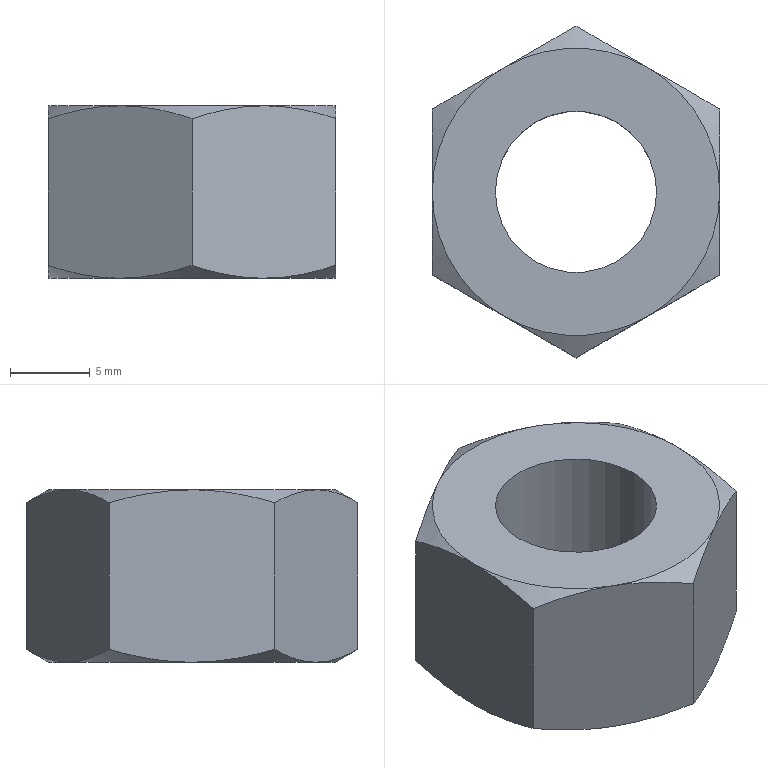Part | SolidWorks | features Cut 2, Extrusion 1 | 1 solid | 22 faces | box 18 x 20.785 x 10.8 mm | volume 2151 mm3 | cone 12 | plane 8 | cylinder 2 | commonest cylinder face diameters 10.106 x2
STEP:
#1=CARTESIAN_POINT('',(-5.053,0.,10.8));
#2=VERTEX_POINT('',#1);
#3=CARTESIAN_POINT('',(5.053,0.,10.8));
#4=VERTEX_POINT('',#3);
#5=CARTESIAN_POINT('',(0.,0.,10.8));
#6=DIRECTION('',(0.,0.,1.));
#7=DIRECTION('',(1.,0.,0.));
#8=AXIS2_PLACEMENT_3D('',#5,#6,#7);
#9=CIRCLE('',#8,5.053);
#10=EDGE_CURVE('',#2,#4,#9,.T.);
#11=ORIENTED_EDGE('',*,*,#10,.T.);
#12=CARTESIAN_POINT('',(5.053,0.,0.));
#13=VERTEX_POINT('',#12);
#14=CARTESIAN_POINT('',(5.053,0.,10.8));
#15=DIRECTION('',(0.,0.,-1.));
#16=VECTOR('',#15,1000.);
#17=LINE('',#14,#16);
#18=EDGE_CURVE('',#4,#13,#17,.T.);
#19=ORIENTED_EDGE('',*,*,#18,.T.);
#20=CARTESIAN_POINT('',(-5.053,0.,0.));
#21=VERTEX_POINT('',#20);
#22=CARTESIAN_POINT('',(0.,0.,0.));
#23=DIRECTION('',(0.,0.,1.));
#24=DIRECTION('',(1.,0.,0.));
#25=AXIS2_PLACEMENT_3D('',#22,#23,#24);
#26=CIRCLE('',#25,5.053);
#27=EDGE_CURVE('',#21,#13,#26,.T.);
#28=ORIENTED_EDGE('',*,*,#27,.F.);
#29=CARTESIAN_POINT('',(-5.053,0.,10.8));
#30=DIRECTION('',(0.,0.,-1.));
#31=VECTOR('',#30,1000.);
#32=LINE('',#29,#31);
#33=EDGE_CURVE('',#2,#21,#32,.T.);
#34=ORIENTED_EDGE('',*,*,#33,.F.);
#35=EDGE_LOOP('',(#11,#19,#28,#34));
#36=FACE_OUTER_BOUND('',#35,.T.);
#37=CARTESIAN_POINT('',(0.,0.,10.8));
#38=DIRECTION('',(0.,0.,-1.));
#39=DIRECTION('',(-1.,0.,0.));
#40=AXIS2_PLACEMENT_3D('',#37,#38,#39);
#41=CYLINDRICAL_SURFACE('',#40,5.053);
#42=ADVANCED_FACE('',(#36),#41,.F.);
#43=CARTESIAN_POINT('',(9.,5.196,9.996));
#44=VERTEX_POINT('',#43);
#45=CARTESIAN_POINT('',(4.5,7.794,10.8));
#46=VERTEX_POINT('',#45);
#47=CARTESIAN_POINT('',(9.,5.196,9.996));
#48=CARTESIAN_POINT('',(8.264,5.621,10.242));
#49=CARTESIAN_POINT('',(7.522,6.049,10.444));
#50=CARTESIAN_POINT('',(6.024,6.914,10.723));
#51=CARTESIAN_POINT('',(5.267,7.352,10.8));
#52=CARTESIAN_POINT('',(4.5,7.794,10.8));
#53=B_SPLINE_CURVE_WITH_KNOTS('',3,(#47,#48,#49,#50,#51,#52),.UNSPECIFIED.,.F.,.F.,(4,2,4),(0.000000238,0.002629,0.005258),.UNSPECIFIED.);
#54=EDGE_CURVE('',#44,#46,#53,.T.);
#55=ORIENTED_EDGE('',*,*,#54,.F.);
#56=CARTESIAN_POINT('',(9.,5.196,0.8038));
#57=VERTEX_POINT('',#56);
#58=CARTESIAN_POINT('',(9.,5.196,10.8));
#59=DIRECTION('',(0.,0.,-1.));
#60=VECTOR('',#59,1000.);
#61=LINE('',#58,#60);
#62=EDGE_CURVE('',#44,#57,#61,.T.);
#63=ORIENTED_EDGE('',*,*,#62,.T.);
#64=CARTESIAN_POINT('',(4.5,7.794,0.));
#65=VERTEX_POINT('',#64);
#66=CARTESIAN_POINT('',(4.5,7.794,0.));
#67=CARTESIAN_POINT('',(4.882,7.574,0.));
#68=CARTESIAN_POINT('',(5.266,7.352,0.019));
#69=CARTESIAN_POINT('',(6.024,6.914,0.09253));
#70=CARTESIAN_POINT('',(6.401,6.697,0.147));
#71=CARTESIAN_POINT('',(7.525,6.048,0.357));
#72=CARTESIAN_POINT('',(8.266,5.62,0.5591));
#73=CARTESIAN_POINT('',(9.,5.196,0.8038));
#74=B_SPLINE_CURVE_WITH_KNOTS('',3,(#66,#67,#68,#69,#70,#71,#72,#73),.UNSPECIFIED.,.F.,.F.,(4,2,2,4),(0.005258,0.006567,0.007877,0.0105),.UNSPECIFIED.);
#75=EDGE_CURVE('',#65,#57,#74,.T.);
#76=ORIENTED_EDGE('',*,*,#75,.F.);
#77=CARTESIAN_POINT('',(0.,10.392,0.8038));
#78=VERTEX_POINT('',#77);
#79=CARTESIAN_POINT('',(0.,10.392,0.8038));
#80=CARTESIAN_POINT('',(0.7361,9.967,0.5585));
#81=CARTESIAN_POINT('',(1.478,9.539,0.3563));
#82=CARTESIAN_POINT('',(2.976,8.674,0.07661));
#83=CARTESIAN_POINT('',(3.733,8.237,0.));
#84=CARTESIAN_POINT('',(4.5,7.794,0.));
#85=B_SPLINE_CURVE_WITH_KNOTS('',3,(#79,#80,#81,#82,#83,#84),.UNSPECIFIED.,.F.,.F.,(4,2,4),(0.000000238,0.002629,0.005258),.UNSPECIFIED.);
#86=EDGE_CURVE('',#78,#65,#85,.T.);
#87=ORIENTED_EDGE('',*,*,#86,.F.);
#88=CARTESIAN_POINT('',(0.,10.392,9.996));
#89=VERTEX_POINT('',#88);
#90=CARTESIAN_POINT('',(0.,10.392,10.8));
#91=DIRECTION('',(0.,0.,-1.));
#92=VECTOR('',#91,1000.);
#93=LINE('',#90,#92);
#94=EDGE_CURVE('',#89,#78,#93,.T.);
#95=ORIENTED_EDGE('',*,*,#94,.F.);
#96=CARTESIAN_POINT('',(4.5,7.794,10.8));
#97=CARTESIAN_POINT('',(4.118,8.015,10.8));
#98=CARTESIAN_POINT('',(3.734,8.236,10.781));
#99=CARTESIAN_POINT('',(2.976,8.674,10.707));
#100=CARTESIAN_POINT('',(2.599,8.892,10.653));
#101=CARTESIAN_POINT('',(1.475,9.541,10.443));
#102=CARTESIAN_POINT('',(0.7343,9.968,10.241));
#103=CARTESIAN_POINT('',(0.,10.392,9.996));
#104=B_SPLINE_CURVE_WITH_KNOTS('',3,(#96,#97,#98,#99,#100,#101,#102,#103),.UNSPECIFIED.,.F.,.F.,(4,2,2,4),(0.005258,0.006567,0.007877,0.0105),.UNSPECIFIED.);
#105=EDGE_CURVE('',#46,#89,#104,.T.);
#106=ORIENTED_EDGE('',*,*,#105,.F.);
#107=EDGE_LOOP('',(#55,#63,#76,#87,#95,#106));
#108=FACE_OUTER_BOUND('',#107,.T.);
#109=CARTESIAN_POINT('',(9.,5.196,10.8));
#110=DIRECTION('',(-0.5,-0.866,0.));
#111=DIRECTION('',(0.866,-0.5,0.));
#112=AXIS2_PLACEMENT_3D('',#109,#110,#111);
#113=PLANE('',#112);
#114=ADVANCED_FACE('',(#108),#113,.F.);
#115=CARTESIAN_POINT('',(-4.5,7.794,10.8));
#116=VERTEX_POINT('',#115);
#117=CARTESIAN_POINT('',(0.,10.392,9.996));
#118=CARTESIAN_POINT('',(-0.7361,9.967,10.242));
#119=CARTESIAN_POINT('',(-1.478,9.539,10.444));
#120=CARTESIAN_POINT('',(-2.976,8.674,10.723));
#121=CARTESIAN_POINT('',(-3.733,8.237,10.8));
#122=CARTESIAN_POINT('',(-4.5,7.794,10.8));
#123=B_SPLINE_CURVE_WITH_KNOTS('',3,(#117,#118,#119,#120,#121,#122),.UNSPECIFIED.,.F.,.F.,(4,2,4),(0.000000238,0.002629,0.005258),.UNSPECIFIED.);
#124=EDGE_CURVE('',#89,#116,#123,.T.);
#125=ORIENTED_EDGE('',*,*,#124,.F.);
#126=ORIENTED_EDGE('',*,*,#94,.T.);
#127=CARTESIAN_POINT('',(-4.5,7.794,0.));
#128=VERTEX_POINT('',#127);
#129=CARTESIAN_POINT('',(-4.5,7.794,0.));
#130=CARTESIAN_POINT('',(-4.118,8.015,0.));
#131=CARTESIAN_POINT('',(-3.734,8.236,0.019));
#132=CARTESIAN_POINT('',(-2.976,8.674,0.09253));
#133=CARTESIAN_POINT('',(-2.599,8.892,0.147));
#134=CARTESIAN_POINT('',(-1.475,9.541,0.357));
#135=CARTESIAN_POINT('',(-0.7343,9.968,0.5591));
#136=CARTESIAN_POINT('',(0.,10.392,0.8038));
#137=B_SPLINE_CURVE_WITH_KNOTS('',3,(#129,#130,#131,#132,#133,#134,#135,#136),.UNSPECIFIED.,.F.,.F.,(4,2,2,4),(0.005258,0.006567,0.007877,0.0105),.UNSPECIFIED.);
#138=EDGE_CURVE('',#128,#78,#137,.T.);
#139=ORIENTED_EDGE('',*,*,#138,.F.);
#140=CARTESIAN_POINT('',(-9.,5.196,0.8038));
#141=VERTEX_POINT('',#140);
#142=CARTESIAN_POINT('',(-9.,5.196,0.8038));
#143=CARTESIAN_POINT('',(-8.264,5.621,0.5585));
#144=CARTESIAN_POINT('',(-7.522,6.049,0.3563));
#145=CARTESIAN_POINT('',(-6.024,6.914,0.07661));
#146=CARTESIAN_POINT('',(-5.267,7.352,0.));
#147=CARTESIAN_POINT('',(-4.5,7.794,0.));
#148=B_SPLINE_CURVE_WITH_KNOTS('',3,(#142,#143,#144,#145,#146,#147),.UNSPECIFIED.,.F.,.F.,(4,2,4),(0.000000238,0.002629,0.005258),.UNSPECIFIED.);
#149=EDGE_CURVE('',#141,#128,#148,.T.);
#150=ORIENTED_EDGE('',*,*,#149,.F.);
#151=CARTESIAN_POINT('',(-9.,5.196,9.996));
#152=VERTEX_POINT('',#151);
#153=CARTESIAN_POINT('',(-9.,5.196,10.8));
#154=DIRECTION('',(0.,0.,-1.));
#155=VECTOR('',#154,1000.);
#156=LINE('',#153,#155);
#157=EDGE_CURVE('',#152,#141,#156,.T.);
#158=ORIENTED_EDGE('',*,*,#157,.F.);
#159=CARTESIAN_POINT('',(-4.5,7.794,10.8));
#160=CARTESIAN_POINT('',(-4.882,7.574,10.8));
#161=CARTESIAN_POINT('',(-5.266,7.352,10.781));
#162=CARTESIAN_POINT('',(-6.024,6.914,10.707));
#163=CARTESIAN_POINT('',(-6.401,6.697,10.653));
#164=CARTESIAN_POINT('',(-7.525,6.048,10.443));
#165=CARTESIAN_POINT('',(-8.266,5.62,10.241));
#166=CARTESIAN_POINT('',(-9.,5.196,9.996));
#167=B_SPLINE_CURVE_WITH_KNOTS('',3,(#159,#160,#161,#162,#163,#164,#165,#166),.UNSPECIFIED.,.F.,.F.,(4,2,2,4),(0.005258,0.006567,0.007877,0.0105),.UNSPECIFIED.);
#168=EDGE_CURVE('',#116,#152,#167,.T.);
#169=ORIENTED_EDGE('',*,*,#168,.F.);
#170=EDGE_LOOP('',(#125,#126,#139,#150,#158,#169));
#171=FACE_OUTER_BOUND('',#170,.T.);
#172=CARTESIAN_POINT('',(0.,10.392,10.8));
#173=DIRECTION('',(0.5,-0.866,0.));
#174=DIRECTION('',(0.866,0.5,0.));
#175=AXIS2_PLACEMENT_3D('',#172,#173,#174);
#176=PLANE('',#175);
#177=ADVANCED_FACE('',(#171),#176,.F.);
#178=CARTESIAN_POINT('',(-9.,0.,10.8));
#179=VERTEX_POINT('',#178);
#180=CARTESIAN_POINT('',(-9.,5.196,9.996));
#181=CARTESIAN_POINT('',(-9.,4.356,10.239));
#182=CARTESIAN_POINT('',(-9.,3.505,10.441));
#183=CARTESIAN_POINT('',(-9.,2.204,10.652));
#184=CARTESIAN_POINT('',(-9.,1.766,10.707));
#185=CARTESIAN_POINT('',(-9.,0.8814,10.781));
#186=CARTESIAN_POINT('',(-9.,0.4397,10.8));
#187=CARTESIAN_POINT('',(-9.,0.,10.8));
#188=B_SPLINE_CURVE_WITH_KNOTS('',3,(#180,#181,#182,#183,#184,#185,#186,#187),.UNSPECIFIED.,.F.,.F.,(4,2,2,4),(0.02958,0.03221,0.03352,0.03484),.UNSPECIFIED.);
#189=EDGE_CURVE('',#152,#179,#188,.T.);
#190=ORIENTED_EDGE('',*,*,#189,.F.);
#191=ORIENTED_EDGE('',*,*,#157,.T.);
#192=CARTESIAN_POINT('',(-9.,0.,0.));
#193=VERTEX_POINT('',#192);
#194=CARTESIAN_POINT('',(-9.,0.,0.));
#195=CARTESIAN_POINT('',(-9.,0.4397,0.));
#196=CARTESIAN_POINT('',(-9.,0.8814,0.01874));
#197=CARTESIAN_POINT('',(-9.,1.766,0.09308));
#198=CARTESIAN_POINT('',(-9.,2.204,0.1481));
#199=CARTESIAN_POINT('',(-9.,3.505,0.3593));
#200=CARTESIAN_POINT('',(-9.,4.356,0.5613));
#201=CARTESIAN_POINT('',(-9.,5.196,0.8038));
#202=B_SPLINE_CURVE_WITH_KNOTS('',3,(#194,#195,#196,#197,#198,#199,#200,#201),.UNSPECIFIED.,.F.,.F.,(4,2,2,4),(0.01478,0.01609,0.01741,0.02004),.UNSPECIFIED.);
#203=EDGE_CURVE('',#193,#141,#202,.T.);
#204=ORIENTED_EDGE('',*,*,#203,.F.);
#205=CARTESIAN_POINT('',(-9.,-5.196,0.8038));
#206=VERTEX_POINT('',#205);
#207=CARTESIAN_POINT('',(-9.,-5.196,0.8038));
#208=CARTESIAN_POINT('',(-9.,-4.35,0.5597));
#209=CARTESIAN_POINT('',(-9.,-3.485,0.3552));
#210=CARTESIAN_POINT('',(-9.,-1.751,0.07559));
#211=CARTESIAN_POINT('',(-9.,-0.8788,0.));
#212=CARTESIAN_POINT('',(-9.,0.,0.));
#213=B_SPLINE_CURVE_WITH_KNOTS('',3,(#207,#208,#209,#210,#211,#212),.UNSPECIFIED.,.F.,.F.,(4,2,4),(0.009518,0.01215,0.01478),.UNSPECIFIED.);
#214=EDGE_CURVE('',#206,#193,#213,.T.);
#215=ORIENTED_EDGE('',*,*,#214,.F.);
#216=CARTESIAN_POINT('',(-9.,-5.196,9.996));
#217=VERTEX_POINT('',#216);
#218=CARTESIAN_POINT('',(-9.,-5.196,10.8));
#219=DIRECTION('',(0.,0.,-1.));
#220=VECTOR('',#219,1000.);
#221=LINE('',#218,#220);
#222=EDGE_CURVE('',#217,#206,#221,.T.);
#223=ORIENTED_EDGE('',*,*,#222,.F.);
#224=CARTESIAN_POINT('',(-9.,0.,10.8));
#225=CARTESIAN_POINT('',(-9.,-0.8788,10.8));
#226=CARTESIAN_POINT('',(-9.,-1.751,10.724));
#227=CARTESIAN_POINT('',(-9.,-3.485,10.445));
#228=CARTESIAN_POINT('',(-9.,-4.35,10.24));
#229=CARTESIAN_POINT('',(-9.,-5.196,9.996));
#230=B_SPLINE_CURVE_WITH_KNOTS('',3,(#224,#225,#226,#227,#228,#229),.UNSPECIFIED.,.F.,.F.,(4,2,4),(0.03484,0.03747,0.0401),.UNSPECIFIED.);
#231=EDGE_CURVE('',#179,#217,#230,.T.);
#232=ORIENTED_EDGE('',*,*,#231,.F.);
#233=EDGE_LOOP('',(#190,#191,#204,#215,#223,#232));
#234=FACE_OUTER_BOUND('',#233,.T.);
#235=CARTESIAN_POINT('',(-9.,5.196,10.8));
#236=DIRECTION('',(1.,0.,0.));
#237=DIRECTION('',(0.,1.,0.));
#238=AXIS2_PLACEMENT_3D('',#235,#236,#237);
#239=PLANE('',#238);
#240=ADVANCED_FACE('',(#234),#239,.F.);
#241=CARTESIAN_POINT('',(-4.5,-7.794,10.8));
#242=VERTEX_POINT('',#241);
#243=CARTESIAN_POINT('',(-9.,-5.196,9.996));
#244=CARTESIAN_POINT('',(-8.264,-5.621,10.242));
#245=CARTESIAN_POINT('',(-7.522,-6.049,10.444));
#246=CARTESIAN_POINT('',(-6.024,-6.914,10.723));
#247=CARTESIAN_POINT('',(-5.267,-7.352,10.8));
#248=CARTESIAN_POINT('',(-4.5,-7.794,10.8));
#249=B_SPLINE_CURVE_WITH_KNOTS('',3,(#243,#244,#245,#246,#247,#248),.UNSPECIFIED.,.F.,.F.,(4,2,4),(0.000000238,0.002629,0.005258),.UNSPECIFIED.);
#250=EDGE_CURVE('',#217,#242,#249,.T.);
#251=ORIENTED_EDGE('',*,*,#250,.F.);
#252=ORIENTED_EDGE('',*,*,#222,.T.);
#253=CARTESIAN_POINT('',(-4.5,-7.794,0.));
#254=VERTEX_POINT('',#253);
#255=CARTESIAN_POINT('',(-4.5,-7.794,0.));
#256=CARTESIAN_POINT('',(-4.882,-7.574,0.));
#257=CARTESIAN_POINT('',(-5.266,-7.352,0.019));
#258=CARTESIAN_POINT('',(-6.024,-6.914,0.09253));
#259=CARTESIAN_POINT('',(-6.401,-6.697,0.147));
#260=CARTESIAN_POINT('',(-7.525,-6.048,0.357));
#261=CARTESIAN_POINT('',(-8.266,-5.62,0.5591));
#262=CARTESIAN_POINT('',(-9.,-5.196,0.8038));
#263=B_SPLINE_CURVE_WITH_KNOTS('',3,(#255,#256,#257,#258,#259,#260,#261,#262),.UNSPECIFIED.,.F.,.F.,(4,2,2,4),(0.005258,0.006567,0.007877,0.0105),.UNSPECIFIED.);
#264=EDGE_CURVE('',#254,#206,#263,.T.);
#265=ORIENTED_EDGE('',*,*,#264,.F.);
#266=CARTESIAN_POINT('',(0.,-10.392,0.8038));
#267=VERTEX_POINT('',#266);
#268=CARTESIAN_POINT('',(0.,-10.392,0.8038));
#269=CARTESIAN_POINT('',(-0.7361,-9.967,0.5585));
#270=CARTESIAN_POINT('',(-1.478,-9.539,0.3563));
#271=CARTESIAN_POINT('',(-2.976,-8.674,0.07661));
#272=CARTESIAN_POINT('',(-3.733,-8.237,0.));
#273=CARTESIAN_POINT('',(-4.5,-7.794,0.));
#274=B_SPLINE_CURVE_WITH_KNOTS('',3,(#268,#269,#270,#271,#272,#273),.UNSPECIFIED.,.F.,.F.,(4,2,4),(0.000000238,0.002629,0.005258),.UNSPECIFIED.);
#275=EDGE_CURVE('',#267,#254,#274,.T.);
#276=ORIENTED_EDGE('',*,*,#275,.F.);
#277=CARTESIAN_POINT('',(0.,-10.392,9.996));
#278=VERTEX_POINT('',#277);
#279=CARTESIAN_POINT('',(0.,-10.392,10.8));
#280=DIRECTION('',(0.,0.,-1.));
#281=VECTOR('',#280,1000.);
#282=LINE('',#279,#281);
#283=EDGE_CURVE('',#278,#267,#282,.T.);
#284=ORIENTED_EDGE('',*,*,#283,.F.);
#285=CARTESIAN_POINT('',(-4.5,-7.794,10.8));
#286=CARTESIAN_POINT('',(-4.118,-8.015,10.8));
#287=CARTESIAN_POINT('',(-3.734,-8.236,10.781));
#288=CARTESIAN_POINT('',(-2.976,-8.674,10.707));
#289=CARTESIAN_POINT('',(-2.599,-8.892,10.653));
#290=CARTESIAN_POINT('',(-1.475,-9.541,10.443));
#291=CARTESIAN_POINT('',(-0.7343,-9.968,10.241));
#292=CARTESIAN_POINT('',(0.,-10.392,9.996));
#293=B_SPLINE_CURVE_WITH_KNOTS('',3,(#285,#286,#287,#288,#289,#290,#291,#292),.UNSPECIFIED.,.F.,.F.,(4,2,2,4),(0.005258,0.006567,0.007877,0.0105),.UNSPECIFIED.);
#294=EDGE_CURVE('',#242,#278,#293,.T.);
#295=ORIENTED_EDGE('',*,*,#294,.F.);
#296=EDGE_LOOP('',(#251,#252,#265,#276,#284,#295));
#297=FACE_OUTER_BOUND('',#296,.T.);
#298=CARTESIAN_POINT('',(-9.,-5.196,10.8));
#299=DIRECTION('',(0.5,0.866,0.));
#300=DIRECTION('',(-0.866,0.5,0.));
#301=AXIS2_PLACEMENT_3D('',#298,#299,#300);
#302=PLANE('',#301);
#303=ADVANCED_FACE('',(#297),#302,.F.);
#304=CARTESIAN_POINT('',(4.5,-7.794,10.8));
#305=VERTEX_POINT('',#304);
#306=CARTESIAN_POINT('',(0.,-10.392,9.996));
#307=CARTESIAN_POINT('',(0.7361,-9.967,10.242));
#308=CARTESIAN_POINT('',(1.478,-9.539,10.444));
#309=CARTESIAN_POINT('',(2.976,-8.674,10.723));
#310=CARTESIAN_POINT('',(3.733,-8.237,10.8));
#311=CARTESIAN_POINT('',(4.5,-7.794,10.8));
#312=B_SPLINE_CURVE_WITH_KNOTS('',3,(#306,#307,#308,#309,#310,#311),.UNSPECIFIED.,.F.,.F.,(4,2,4),(0.000000238,0.002629,0.005258),.UNSPECIFIED.);
#313=EDGE_CURVE('',#278,#305,#312,.T.);
#314=ORIENTED_EDGE('',*,*,#313,.F.);
#315=ORIENTED_EDGE('',*,*,#283,.T.);
#316=CARTESIAN_POINT('',(4.5,-7.794,0.));
#317=VERTEX_POINT('',#316);
#318=CARTESIAN_POINT('',(4.5,-7.794,0.));
#319=CARTESIAN_POINT('',(4.118,-8.015,0.));
#320=CARTESIAN_POINT('',(3.734,-8.236,0.019));
#321=CARTESIAN_POINT('',(2.976,-8.674,0.09253));
#322=CARTESIAN_POINT('',(2.599,-8.892,0.147));
#323=CARTESIAN_POINT('',(1.475,-9.541,0.357));
#324=CARTESIAN_POINT('',(0.7343,-9.968,0.5591));
#325=CARTESIAN_POINT('',(0.,-10.392,0.8038));
#326=B_SPLINE_CURVE_WITH_KNOTS('',3,(#318,#319,#320,#321,#322,#323,#324,#325),.UNSPECIFIED.,.F.,.F.,(4,2,2,4),(0.005258,0.006567,0.007877,0.0105),.UNSPECIFIED.);
#327=EDGE_CURVE('',#317,#267,#326,.T.);
#328=ORIENTED_EDGE('',*,*,#327,.F.);
#329=CARTESIAN_POINT('',(9.,-5.196,0.8038));
#330=VERTEX_POINT('',#329);
#331=CARTESIAN_POINT('',(9.,-5.196,0.8038));
#332=CARTESIAN_POINT('',(8.264,-5.621,0.5585));
#333=CARTESIAN_POINT('',(7.522,-6.049,0.3563));
#334=CARTESIAN_POINT('',(6.024,-6.914,0.07661));
#335=CARTESIAN_POINT('',(5.267,-7.352,0.));
#336=CARTESIAN_POINT('',(4.5,-7.794,0.));
#337=B_SPLINE_CURVE_WITH_KNOTS('',3,(#331,#332,#333,#334,#335,#336),.UNSPECIFIED.,.F.,.F.,(4,2,4),(0.000000238,0.002629,0.005258),.UNSPECIFIED.);
#338=EDGE_CURVE('',#330,#317,#337,.T.);
#339=ORIENTED_EDGE('',*,*,#338,.F.);
#340=CARTESIAN_POINT('',(9.,-5.196,9.996));
#341=VERTEX_POINT('',#340);
#342=CARTESIAN_POINT('',(9.,-5.196,10.8));
#343=DIRECTION('',(0.,0.,-1.));
#344=VECTOR('',#343,1000.);
#345=LINE('',#342,#344);
#346=EDGE_CURVE('',#341,#330,#345,.T.);
#347=ORIENTED_EDGE('',*,*,#346,.F.);
#348=CARTESIAN_POINT('',(4.5,-7.794,10.8));
#349=CARTESIAN_POINT('',(4.882,-7.574,10.8));
#350=CARTESIAN_POINT('',(5.266,-7.352,10.781));
#351=CARTESIAN_POINT('',(6.024,-6.914,10.707));
#352=CARTESIAN_POINT('',(6.401,-6.697,10.653));
#353=CARTESIAN_POINT('',(7.525,-6.048,10.443));
#354=CARTESIAN_POINT('',(8.266,-5.62,10.241));
#355=CARTESIAN_POINT('',(9.,-5.196,9.996));
#356=B_SPLINE_CURVE_WITH_KNOTS('',3,(#348,#349,#350,#351,#352,#353,#354,#355),.UNSPECIFIED.,.F.,.F.,(4,2,2,4),(0.005258,0.006567,0.007877,0.0105),.UNSPECIFIED.);
#357=EDGE_CURVE('',#305,#341,#356,.T.);
#358=ORIENTED_EDGE('',*,*,#357,.F.);
#359=EDGE_LOOP('',(#314,#315,#328,#339,#347,#358));
#360=FACE_OUTER_BOUND('',#359,.T.);
#361=CARTESIAN_POINT('',(0.,-10.392,10.8));
#362=DIRECTION('',(-0.5,0.866,0.));
#363=DIRECTION('',(-0.866,-0.5,0.));
#364=AXIS2_PLACEMENT_3D('',#361,#362,#363);
#365=PLANE('',#364);
#366=ADVANCED_FACE('',(#360),#365,.F.);
#367=CARTESIAN_POINT('',(9.,0.,10.8));
#368=VERTEX_POINT('',#367);
#369=CARTESIAN_POINT('',(9.,-5.196,9.996));
#370=CARTESIAN_POINT('',(9.,-4.35,10.24));
#371=CARTESIAN_POINT('',(9.,-3.485,10.445));
#372=CARTESIAN_POINT('',(9.,-1.751,10.724));
#373=CARTESIAN_POINT('',(9.,-0.8788,10.8));
#374=CARTESIAN_POINT('',(9.,0.,10.8));
#375=B_SPLINE_CURVE_WITH_KNOTS('',3,(#369,#370,#371,#372,#373,#374),.UNSPECIFIED.,.F.,.F.,(4,2,4),(0.009518,0.01215,0.01478),.UNSPECIFIED.);
#376=EDGE_CURVE('',#341,#368,#375,.T.);
#377=ORIENTED_EDGE('',*,*,#376,.F.);
#378=ORIENTED_EDGE('',*,*,#346,.T.);
#379=CARTESIAN_POINT('',(9.,0.,0.));
#380=VERTEX_POINT('',#379);
#381=CARTESIAN_POINT('',(9.,0.,0.));
#382=CARTESIAN_POINT('',(9.,-0.8788,0.));
#383=CARTESIAN_POINT('',(9.,-1.751,0.07559));
#384=CARTESIAN_POINT('',(9.,-3.485,0.3552));
#385=CARTESIAN_POINT('',(9.,-4.35,0.5597));
#386=CARTESIAN_POINT('',(9.,-5.196,0.8038));
#387=B_SPLINE_CURVE_WITH_KNOTS('',3,(#381,#382,#383,#384,#385,#386),.UNSPECIFIED.,.F.,.F.,(4,2,4),(0.03484,0.03747,0.0401),.UNSPECIFIED.);
#388=EDGE_CURVE('',#380,#330,#387,.T.);
#389=ORIENTED_EDGE('',*,*,#388,.F.);
#390=CARTESIAN_POINT('',(9.,5.196,0.8038));
#391=CARTESIAN_POINT('',(9.,4.356,0.5613));
#392=CARTESIAN_POINT('',(9.,3.505,0.3593));
#393=CARTESIAN_POINT('',(9.,2.204,0.1481));
#394=CARTESIAN_POINT('',(9.,1.766,0.09308));
#395=CARTESIAN_POINT('',(9.,0.8814,0.01874));
#396=CARTESIAN_POINT('',(9.,0.4397,0.));
#397=CARTESIAN_POINT('',(9.,0.,0.));
#398=B_SPLINE_CURVE_WITH_KNOTS('',3,(#390,#391,#392,#393,#394,#395,#396,#397),.UNSPECIFIED.,.F.,.F.,(4,2,2,4),(0.02958,0.03221,0.03352,0.03484),.UNSPECIFIED.);
#399=EDGE_CURVE('',#57,#380,#398,.T.);
#400=ORIENTED_EDGE('',*,*,#399,.F.);
#401=ORIENTED_EDGE('',*,*,#62,.F.);
#402=CARTESIAN_POINT('',(9.,0.,10.8));
#403=CARTESIAN_POINT('',(9.,0.4397,10.8));
#404=CARTESIAN_POINT('',(9.,0.8814,10.781));
#405=CARTESIAN_POINT('',(9.,1.766,10.707));
#406=CARTESIAN_POINT('',(9.,2.204,10.652));
#407=CARTESIAN_POINT('',(9.,3.505,10.441));
#408=CARTESIAN_POINT('',(9.,4.356,10.239));
#409=CARTESIAN_POINT('',(9.,5.196,9.996));
#410=B_SPLINE_CURVE_WITH_KNOTS('',3,(#402,#403,#404,#405,#406,#407,#408,#409),.UNSPECIFIED.,.F.,.F.,(4,2,2,4),(0.01478,0.01609,0.01741,0.02004),.UNSPECIFIED.);
#411=EDGE_CURVE('',#368,#44,#410,.T.);
#412=ORIENTED_EDGE('',*,*,#411,.F.);
#413=EDGE_LOOP('',(#377,#378,#389,#400,#401,#412));
#414=FACE_OUTER_BOUND('',#413,.T.);
#415=CARTESIAN_POINT('',(9.,-5.196,10.8));
#416=DIRECTION('',(-1.,0.,0.));
#417=DIRECTION('',(0.,-1.,0.));
#418=AXIS2_PLACEMENT_3D('',#415,#416,#417);
#419=PLANE('',#418);
#420=ADVANCED_FACE('',(#414),#419,.F.);
#421=ORIENTED_EDGE('',*,*,#10,.F.);
#422=CARTESIAN_POINT('',(0.,0.,10.8));
#423=DIRECTION('',(0.,0.,1.));
#424=DIRECTION('',(1.,0.,0.));
#425=AXIS2_PLACEMENT_3D('',#422,#423,#424);
#426=CIRCLE('',#425,5.053);
#427=EDGE_CURVE('',#4,#2,#426,.T.);
#428=ORIENTED_EDGE('',*,*,#427,.F.);
#429=EDGE_LOOP('',(#421,#428));
#430=FACE_BOUND('',#429,.T.);
#431=CARTESIAN_POINT('',(0.,0.,10.8));
#432=DIRECTION('',(0.,0.,1.));
#433=DIRECTION('',(1.,0.,0.));
#434=AXIS2_PLACEMENT_3D('',#431,#432,#433);
#435=CIRCLE('',#434,9.);
#436=EDGE_CURVE('',#305,#368,#435,.T.);
#437=ORIENTED_EDGE('',*,*,#436,.T.);
#438=CARTESIAN_POINT('',(0.,0.,10.8));
#439=DIRECTION('',(0.,0.,1.));
#440=DIRECTION('',(1.,0.,0.));
#441=AXIS2_PLACEMENT_3D('',#438,#439,#440);
#442=CIRCLE('',#441,9.);
#443=EDGE_CURVE('',#368,#46,#442,.T.);
#444=ORIENTED_EDGE('',*,*,#443,.T.);
#445=CARTESIAN_POINT('',(0.,0.,10.8));
#446=DIRECTION('',(0.,0.,1.));
#447=DIRECTION('',(1.,0.,0.));
#448=AXIS2_PLACEMENT_3D('',#445,#446,#447);
#449=CIRCLE('',#448,9.);
#450=EDGE_CURVE('',#46,#116,#449,.T.);
#451=ORIENTED_EDGE('',*,*,#450,.T.);
#452=CARTESIAN_POINT('',(0.,0.,10.8));
#453=DIRECTION('',(0.,0.,1.));
#454=DIRECTION('',(1.,0.,0.));
#455=AXIS2_PLACEMENT_3D('',#452,#453,#454);
#456=CIRCLE('',#455,9.);
#457=EDGE_CURVE('',#116,#179,#456,.T.);
#458=ORIENTED_EDGE('',*,*,#457,.T.);
#459=CARTESIAN_POINT('',(0.,0.,10.8));
#460=DIRECTION('',(0.,0.,1.));
#461=DIRECTION('',(1.,0.,0.));
#462=AXIS2_PLACEMENT_3D('',#459,#460,#461);
#463=CIRCLE('',#462,9.);
#464=EDGE_CURVE('',#179,#242,#463,.T.);
#465=ORIENTED_EDGE('',*,*,#464,.T.);
#466=CARTESIAN_POINT('',(0.,0.,10.8));
#467=DIRECTION('',(0.,0.,1.));
#468=DIRECTION('',(1.,0.,0.));
#469=AXIS2_PLACEMENT_3D('',#466,#467,#468);
#470=CIRCLE('',#469,9.);
#471=EDGE_CURVE('',#242,#305,#470,.T.);
#472=ORIENTED_EDGE('',*,*,#471,.T.);
#473=EDGE_LOOP('',(#437,#444,#451,#458,#465,#472));
#474=FACE_OUTER_BOUND('',#473,.T.);
#475=CARTESIAN_POINT('',(-9.,15.588,10.8));
#476=DIRECTION('',(0.,0.,1.));
#477=DIRECTION('',(1.,0.,0.));
#478=AXIS2_PLACEMENT_3D('',#475,#476,#477);
#479=PLANE('',#478);
#480=ADVANCED_FACE('',(#430,#474),#479,.T.);
#481=ORIENTED_EDGE('',*,*,#27,.T.);
#482=CARTESIAN_POINT('',(0.,0.,0.));
#483=DIRECTION('',(0.,0.,1.));
#484=DIRECTION('',(1.,0.,0.));
#485=AXIS2_PLACEMENT_3D('',#482,#483,#484);
#486=CIRCLE('',#485,5.053);
#487=EDGE_CURVE('',#13,#21,#486,.T.);
#488=ORIENTED_EDGE('',*,*,#487,.T.);
#489=EDGE_LOOP('',(#481,#488));
#490=FACE_BOUND('',#489,.T.);
#491=CARTESIAN_POINT('',(0.,0.,0.));
#492=DIRECTION('',(0.,0.,-1.));
#493=DIRECTION('',(-1.,0.,0.));
#494=AXIS2_PLACEMENT_3D('',#491,#492,#493);
#495=CIRCLE('',#494,9.);
#496=EDGE_CURVE('',#65,#380,#495,.T.);
#497=ORIENTED_EDGE('',*,*,#496,.T.);
#498=CARTESIAN_POINT('',(0.,0.,0.));
#499=DIRECTION('',(0.,0.,-1.));
#500=DIRECTION('',(-1.,0.,0.));
#501=AXIS2_PLACEMENT_3D('',#498,#499,#500);
#502=CIRCLE('',#501,9.);
#503=EDGE_CURVE('',#380,#317,#502,.T.);
#504=ORIENTED_EDGE('',*,*,#503,.T.);
#505=CARTESIAN_POINT('',(0.,0.,0.));
#506=DIRECTION('',(0.,0.,-1.));
#507=DIRECTION('',(-1.,0.,0.));
#508=AXIS2_PLACEMENT_3D('',#505,#506,#507);
#509=CIRCLE('',#508,9.);
#510=EDGE_CURVE('',#317,#254,#509,.T.);
#511=ORIENTED_EDGE('',*,*,#510,.T.);
#512=CARTESIAN_POINT('',(0.,0.,0.));
#513=DIRECTION('',(0.,0.,-1.));
#514=DIRECTION('',(-1.,0.,0.));
#515=AXIS2_PLACEMENT_3D('',#512,#513,#514);
#516=CIRCLE('',#515,9.);
#517=EDGE_CURVE('',#254,#193,#516,.T.);
#518=ORIENTED_EDGE('',*,*,#517,.T.);
#519=CARTESIAN_POINT('',(0.,0.,0.));
#520=DIRECTION('',(0.,0.,-1.));
#521=DIRECTION('',(-1.,0.,0.));
#522=AXIS2_PLACEMENT_3D('',#519,#520,#521);
#523=CIRCLE('',#522,9.);
#524=EDGE_CURVE('',#193,#128,#523,.T.);
#525=ORIENTED_EDGE('',*,*,#524,.T.);
#526=CARTESIAN_POINT('',(0.,0.,0.));
#527=DIRECTION('',(0.,0.,-1.));
#528=DIRECTION('',(-1.,0.,0.));
#529=AXIS2_PLACEMENT_3D('',#526,#527,#528);
#530=CIRCLE('',#529,9.);
#531=EDGE_CURVE('',#128,#65,#530,.T.);
#532=ORIENTED_EDGE('',*,*,#531,.T.);
#533=EDGE_LOOP('',(#497,#504,#511,#518,#525,#532));
#534=FACE_OUTER_BOUND('',#533,.T.);
#535=CARTESIAN_POINT('',(-9.,15.588,0.));
#536=DIRECTION('',(0.,0.,1.));
#537=DIRECTION('',(1.,0.,0.));
#538=AXIS2_PLACEMENT_3D('',#535,#536,#537);
#539=PLANE('',#538);
#540=ADVANCED_FACE('',(#490,#534),#539,.F.);
#541=ORIENTED_EDGE('',*,*,#18,.F.);
#542=ORIENTED_EDGE('',*,*,#427,.T.);
#543=ORIENTED_EDGE('',*,*,#33,.T.);
#544=ORIENTED_EDGE('',*,*,#487,.F.);
#545=EDGE_LOOP('',(#541,#542,#543,#544));
#546=FACE_OUTER_BOUND('',#545,.T.);
#547=CARTESIAN_POINT('',(0.,0.,10.8));
#548=DIRECTION('',(0.,0.,-1.));
#549=DIRECTION('',(-1.,0.,0.));
#550=AXIS2_PLACEMENT_3D('',#547,#548,#549);
#551=CYLINDRICAL_SURFACE('',#550,5.053);
#552=ADVANCED_FACE('',(#546),#551,.F.);
#553=ORIENTED_EDGE('',*,*,#338,.T.);
#554=ORIENTED_EDGE('',*,*,#503,.F.);
#555=ORIENTED_EDGE('',*,*,#388,.T.);
#556=EDGE_LOOP('',(#553,#554,#555));
#557=FACE_OUTER_BOUND('',#556,.T.);
#558=CARTESIAN_POINT('',(0.,0.,0.));
#559=DIRECTION('',(0.,0.,1.));
#560=DIRECTION('',(-1.,0.,0.));
#561=AXIS2_PLACEMENT_3D('',#558,#559,#560);
#562=CONICAL_SURFACE('',#561,9.,1.047);
#563=ADVANCED_FACE('',(#557),#562,.T.);
#564=ORIENTED_EDGE('',*,*,#75,.T.);
#565=ORIENTED_EDGE('',*,*,#399,.T.);
#566=ORIENTED_EDGE('',*,*,#496,.F.);
#567=EDGE_LOOP('',(#564,#565,#566));
#568=FACE_OUTER_BOUND('',#567,.T.);
#569=CARTESIAN_POINT('',(0.,0.,0.));
#570=DIRECTION('',(0.,0.,1.));
#571=DIRECTION('',(-1.,0.,0.));
#572=AXIS2_PLACEMENT_3D('',#569,#570,#571);
#573=CONICAL_SURFACE('',#572,9.,1.047);
#574=ADVANCED_FACE('',(#568),#573,.T.);
#575=ORIENTED_EDGE('',*,*,#275,.T.);
#576=ORIENTED_EDGE('',*,*,#510,.F.);
#577=ORIENTED_EDGE('',*,*,#327,.T.);
#578=EDGE_LOOP('',(#575,#576,#577));
#579=FACE_OUTER_BOUND('',#578,.T.);
#580=CARTESIAN_POINT('',(0.,0.,0.));
#581=DIRECTION('',(0.,0.,1.));
#582=DIRECTION('',(-1.,0.,0.));
#583=AXIS2_PLACEMENT_3D('',#580,#581,#582);
#584=CONICAL_SURFACE('',#583,9.,1.047);
#585=ADVANCED_FACE('',(#579),#584,.T.);
#586=ORIENTED_EDGE('',*,*,#214,.T.);
#587=ORIENTED_EDGE('',*,*,#517,.F.);
#588=ORIENTED_EDGE('',*,*,#264,.T.);
#589=EDGE_LOOP('',(#586,#587,#588));
#590=FACE_OUTER_BOUND('',#589,.T.);
#591=CARTESIAN_POINT('',(0.,0.,0.));
#592=DIRECTION('',(0.,0.,1.));
#593=DIRECTION('',(-1.,0.,0.));
#594=AXIS2_PLACEMENT_3D('',#591,#592,#593);
#595=CONICAL_SURFACE('',#594,9.,1.047);
#596=ADVANCED_FACE('',(#590),#595,.T.);
#597=ORIENTED_EDGE('',*,*,#203,.T.);
#598=ORIENTED_EDGE('',*,*,#149,.T.);
#599=ORIENTED_EDGE('',*,*,#524,.F.);
#600=EDGE_LOOP('',(#597,#598,#599));
#601=FACE_OUTER_BOUND('',#600,.T.);
#602=CARTESIAN_POINT('',(0.,0.,0.));
#603=DIRECTION('',(0.,0.,1.));
#604=DIRECTION('',(-1.,0.,0.));
#605=AXIS2_PLACEMENT_3D('',#602,#603,#604);
#606=CONICAL_SURFACE('',#605,9.,1.047);
#607=ADVANCED_FACE('',(#601),#606,.T.);
#608=ORIENTED_EDGE('',*,*,#138,.T.);
#609=ORIENTED_EDGE('',*,*,#86,.T.);
#610=ORIENTED_EDGE('',*,*,#531,.F.);
#611=EDGE_LOOP('',(#608,#609,#610));
#612=FACE_OUTER_BOUND('',#611,.T.);
#613=CARTESIAN_POINT('',(0.,0.,0.));
#614=DIRECTION('',(0.,0.,1.));
#615=DIRECTION('',(-1.,0.,0.));
#616=AXIS2_PLACEMENT_3D('',#613,#614,#615);
#617=CONICAL_SURFACE('',#616,9.,1.047);
#618=ADVANCED_FACE('',(#612),#617,.T.);
#619=ORIENTED_EDGE('',*,*,#357,.T.);
#620=ORIENTED_EDGE('',*,*,#376,.T.);
#621=ORIENTED_EDGE('',*,*,#436,.F.);
#622=EDGE_LOOP('',(#619,#620,#621));
#623=FACE_OUTER_BOUND('',#622,.T.);
#624=CARTESIAN_POINT('',(0.,0.,10.8));
#625=DIRECTION('',(0.,0.,-1.));
#626=DIRECTION('',(1.,0.,0.));
#627=AXIS2_PLACEMENT_3D('',#624,#625,#626);
#628=CONICAL_SURFACE('',#627,9.,1.047);
#629=ADVANCED_FACE('',(#623),#628,.T.);
#630=ORIENTED_EDGE('',*,*,#294,.T.);
#631=ORIENTED_EDGE('',*,*,#313,.T.);
#632=ORIENTED_EDGE('',*,*,#471,.F.);
#633=EDGE_LOOP('',(#630,#631,#632));
#634=FACE_OUTER_BOUND('',#633,.T.);
#635=CARTESIAN_POINT('',(0.,0.,10.8));
#636=DIRECTION('',(0.,0.,-1.));
#637=DIRECTION('',(1.,0.,0.));
#638=AXIS2_PLACEMENT_3D('',#635,#636,#637);
#639=CONICAL_SURFACE('',#638,9.,1.047);
#640=ADVANCED_FACE('',(#634),#639,.T.);
#641=ORIENTED_EDGE('',*,*,#231,.T.);
#642=ORIENTED_EDGE('',*,*,#250,.T.);
#643=ORIENTED_EDGE('',*,*,#464,.F.);
#644=EDGE_LOOP('',(#641,#642,#643));
#645=FACE_OUTER_BOUND('',#644,.T.);
#646=CARTESIAN_POINT('',(0.,0.,10.8));
#647=DIRECTION('',(0.,0.,-1.));
#648=DIRECTION('',(1.,0.,0.));
#649=AXIS2_PLACEMENT_3D('',#646,#647,#648);
#650=CONICAL_SURFACE('',#649,9.,1.047);
#651=ADVANCED_FACE('',(#645),#650,.T.);
#652=ORIENTED_EDGE('',*,*,#168,.T.);
#653=ORIENTED_EDGE('',*,*,#189,.T.);
#654=ORIENTED_EDGE('',*,*,#457,.F.);
#655=EDGE_LOOP('',(#652,#653,#654));
#656=FACE_OUTER_BOUND('',#655,.T.);
#657=CARTESIAN_POINT('',(0.,0.,10.8));
#658=DIRECTION('',(0.,0.,-1.));
#659=DIRECTION('',(1.,0.,0.));
#660=AXIS2_PLACEMENT_3D('',#657,#658,#659);
#661=CONICAL_SURFACE('',#660,9.,1.047);
#662=ADVANCED_FACE('',(#656),#661,.T.);
#663=ORIENTED_EDGE('',*,*,#105,.T.);
#664=ORIENTED_EDGE('',*,*,#124,.T.);
#665=ORIENTED_EDGE('',*,*,#450,.F.);
#666=EDGE_LOOP('',(#663,#664,#665));
#667=FACE_OUTER_BOUND('',#666,.T.);
#668=CARTESIAN_POINT('',(0.,0.,10.8));
#669=DIRECTION('',(0.,0.,-1.));
#670=DIRECTION('',(1.,0.,0.));
#671=AXIS2_PLACEMENT_3D('',#668,#669,#670);
#672=CONICAL_SURFACE('',#671,9.,1.047);
#673=ADVANCED_FACE('',(#667),#672,.T.);
#674=ORIENTED_EDGE('',*,*,#54,.T.);
#675=ORIENTED_EDGE('',*,*,#443,.F.);
#676=ORIENTED_EDGE('',*,*,#411,.T.);
#677=EDGE_LOOP('',(#674,#675,#676));
#678=FACE_OUTER_BOUND('',#677,.T.);
#679=CARTESIAN_POINT('',(0.,0.,10.8));
#680=DIRECTION('',(0.,0.,-1.));
#681=DIRECTION('',(1.,0.,0.));
#682=AXIS2_PLACEMENT_3D('',#679,#680,#681);
#683=CONICAL_SURFACE('',#682,9.,1.047);
#684=ADVANCED_FACE('',(#678),#683,.T.);
#685=CLOSED_SHELL('',(#42,#114,#177,#240,#303,#366,#420,#480,#540,#552,#563,#574,#585,#596,#607,#618,#629,#640,#651,#662,#673,#684));
#686=MANIFOLD_SOLID_BREP('',#685);
#687=CARTESIAN_POINT('',(0.,0.,0.));
#688=DIRECTION('',(0.,0.,1.));
#689=DIRECTION('',(1.,0.,0.));
#690=AXIS2_PLACEMENT_3D('',#687,#688,#689);
#691=(LENGTH_UNIT()NAMED_UNIT(*)SI_UNIT(.MILLI.,.METRE.));
#692=UNCERTAINTY_MEASURE_WITH_UNIT(LENGTH_MEASURE(0.00001),#691,'','');
#693=(NAMED_UNIT(*)PLANE_ANGLE_UNIT()SI_UNIT($,.RADIAN.));
#694=(NAMED_UNIT(*)SI_UNIT($,.STERADIAN.)SOLID_ANGLE_UNIT());
#695=(GEOMETRIC_REPRESENTATION_CONTEXT(3)GLOBAL_UNCERTAINTY_ASSIGNED_CONTEXT((#692))GLOBAL_UNIT_ASSIGNED_CONTEXT((#691,#693,#694))REPRESENTATION_CONTEXT('',''));
#696=ADVANCED_BREP_SHAPE_REPRESENTATION('',(#686,#690),#695);